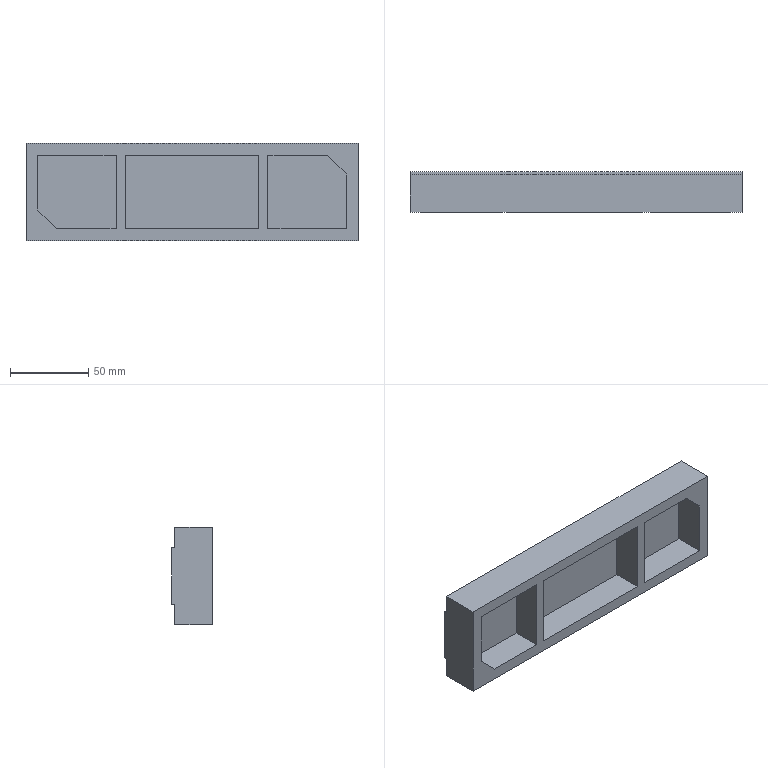Part | SolidWorks | features ICE 2, Extrusion 1, Rib 1, Shell 1 | 1 solid | 27 faces | box 212 x 26 x 62 mm | volume 172526 mm3 | plane 27
STEP:
#1=CARTESIAN_POINT('',(-86.5,18.5,-23.5));
#2=VERTEX_POINT('',#1);
#3=CARTESIAN_POINT('',(-86.5,0.,-23.5));
#4=VERTEX_POINT('',#3);
#5=CARTESIAN_POINT('',(-86.5,500000.,-23.5));
#6=DIRECTION('',(0.,-1.,0.));
#7=VECTOR('',#6,1000.);
#8=LINE('',#5,#7);
#9=EDGE_CURVE('',#2,#4,#8,.T.);
#10=ORIENTED_EDGE('',*,*,#9,.T.);
#11=CARTESIAN_POINT('',(-48.5,0.,-23.5));
#12=VERTEX_POINT('',#11);
#13=CARTESIAN_POINT('',(0.,0.,-23.5));
#14=DIRECTION('',(-1.,0.,0.));
#15=VECTOR('',#14,1000.);
#16=LINE('',#13,#15);
#17=EDGE_CURVE('',#12,#4,#16,.T.);
#18=ORIENTED_EDGE('',*,*,#17,.F.);
#19=CARTESIAN_POINT('',(-48.5,18.5,-23.5));
#20=VERTEX_POINT('',#19);
#21=CARTESIAN_POINT('',(-48.5,0.,-23.5));
#22=DIRECTION('',(0.,1.,0.));
#23=VECTOR('',#22,1000.);
#24=LINE('',#21,#23);
#25=EDGE_CURVE('',#12,#20,#24,.T.);
#26=ORIENTED_EDGE('',*,*,#25,.T.);
#27=CARTESIAN_POINT('',(0.,18.5,-23.5));
#28=DIRECTION('',(-1.,0.,0.));
#29=VECTOR('',#28,1000.);
#30=LINE('',#27,#29);
#31=EDGE_CURVE('',#20,#2,#30,.T.);
#32=ORIENTED_EDGE('',*,*,#31,.T.);
#33=EDGE_LOOP('',(#10,#18,#26,#32));
#34=FACE_OUTER_BOUND('',#33,.T.);
#35=CARTESIAN_POINT('',(-106.,26.,-23.5));
#36=DIRECTION('',(0.,0.,1.));
#37=DIRECTION('',(1.,0.,0.));
#38=AXIS2_PLACEMENT_3D('',#35,#36,#37);
#39=PLANE('',#38);
#40=ADVANCED_FACE('',(#34),#39,.T.);
#41=CARTESIAN_POINT('',(-98.5,18.5,23.5));
#42=VERTEX_POINT('',#41);
#43=CARTESIAN_POINT('',(-48.5,18.5,23.5));
#44=VERTEX_POINT('',#43);
#45=CARTESIAN_POINT('',(0.,18.5,23.5));
#46=DIRECTION('',(1.,0.,0.));
#47=VECTOR('',#46,1000.);
#48=LINE('',#45,#47);
#49=EDGE_CURVE('',#42,#44,#48,.T.);
#50=ORIENTED_EDGE('',*,*,#49,.T.);
#51=CARTESIAN_POINT('',(-48.5,0.,23.5));
#52=VERTEX_POINT('',#51);
#53=CARTESIAN_POINT('',(-48.5,26.,23.5));
#54=DIRECTION('',(0.,-1.,0.));
#55=VECTOR('',#54,1000.);
#56=LINE('',#53,#55);
#57=EDGE_CURVE('',#44,#52,#56,.T.);
#58=ORIENTED_EDGE('',*,*,#57,.T.);
#59=CARTESIAN_POINT('',(-98.5,0.,23.5));
#60=VERTEX_POINT('',#59);
#61=CARTESIAN_POINT('',(0.,0.,23.5));
#62=DIRECTION('',(1.,0.,0.));
#63=VECTOR('',#62,1000.);
#64=LINE('',#61,#63);
#65=EDGE_CURVE('',#60,#52,#64,.T.);
#66=ORIENTED_EDGE('',*,*,#65,.F.);
#67=CARTESIAN_POINT('',(-98.5,26.,23.5));
#68=DIRECTION('',(0.,-1.,0.));
#69=VECTOR('',#68,1000.);
#70=LINE('',#67,#69);
#71=EDGE_CURVE('',#42,#60,#70,.T.);
#72=ORIENTED_EDGE('',*,*,#71,.F.);
#73=EDGE_LOOP('',(#50,#58,#66,#72));
#74=FACE_OUTER_BOUND('',#73,.T.);
#75=CARTESIAN_POINT('',(-106.,26.,23.5));
#76=DIRECTION('',(0.,0.,-1.));
#77=DIRECTION('',(-1.,0.,0.));
#78=AXIS2_PLACEMENT_3D('',#75,#76,#77);
#79=PLANE('',#78);
#80=ADVANCED_FACE('',(#74),#79,.T.);
#81=CARTESIAN_POINT('',(-98.5,18.5,-11.5));
#82=VERTEX_POINT('',#81);
#83=CARTESIAN_POINT('',(-98.5,18.5,-11.5));
#84=DIRECTION('',(0.7071,0.,-0.7071));
#85=VECTOR('',#84,1000.);
#86=LINE('',#83,#85);
#87=EDGE_CURVE('',#82,#2,#86,.T.);
#88=ORIENTED_EDGE('',*,*,#87,.T.);
#89=ORIENTED_EDGE('',*,*,#31,.F.);
#90=CARTESIAN_POINT('',(-48.5,18.5,0.));
#91=DIRECTION('',(0.,0.,1.));
#92=VECTOR('',#91,1000.);
#93=LINE('',#90,#92);
#94=EDGE_CURVE('',#20,#44,#93,.T.);
#95=ORIENTED_EDGE('',*,*,#94,.T.);
#96=ORIENTED_EDGE('',*,*,#49,.F.);
#97=CARTESIAN_POINT('',(-98.5,18.5,0.));
#98=DIRECTION('',(0.,0.,1.));
#99=VECTOR('',#98,1000.);
#100=LINE('',#97,#99);
#101=EDGE_CURVE('',#82,#42,#100,.T.);
#102=ORIENTED_EDGE('',*,*,#101,.F.);
#103=EDGE_LOOP('',(#88,#89,#95,#96,#102));
#104=FACE_OUTER_BOUND('',#103,.T.);
#105=CARTESIAN_POINT('',(0.,18.5,0.));
#106=DIRECTION('',(0.,-1.,0.));
#107=DIRECTION('',(0.,0.,-1.));
#108=AXIS2_PLACEMENT_3D('',#105,#106,#107);
#109=PLANE('',#108);
#110=ADVANCED_FACE('',(#104),#109,.T.);
#111=CARTESIAN_POINT('',(-42.5,0.,-23.5));
#112=VERTEX_POINT('',#111);
#113=CARTESIAN_POINT('',(-42.5,18.5,-23.5));
#114=VERTEX_POINT('',#113);
#115=CARTESIAN_POINT('',(-42.5,0.,-23.5));
#116=DIRECTION('',(0.,1.,0.));
#117=VECTOR('',#116,1000.);
#118=LINE('',#115,#117);
#119=EDGE_CURVE('',#112,#114,#118,.T.);
#120=ORIENTED_EDGE('',*,*,#119,.F.);
#121=CARTESIAN_POINT('',(42.5,0.,-23.5));
#122=VERTEX_POINT('',#121);
#123=CARTESIAN_POINT('',(0.,0.,-23.5));
#124=DIRECTION('',(-1.,0.,0.));
#125=VECTOR('',#124,1000.);
#126=LINE('',#123,#125);
#127=EDGE_CURVE('',#122,#112,#126,.T.);
#128=ORIENTED_EDGE('',*,*,#127,.F.);
#129=CARTESIAN_POINT('',(42.5,18.5,-23.5));
#130=VERTEX_POINT('',#129);
#131=CARTESIAN_POINT('',(42.5,0.,-23.5));
#132=DIRECTION('',(0.,1.,0.));
#133=VECTOR('',#132,1000.);
#134=LINE('',#131,#133);
#135=EDGE_CURVE('',#122,#130,#134,.T.);
#136=ORIENTED_EDGE('',*,*,#135,.T.);
#137=CARTESIAN_POINT('',(0.,18.5,-23.5));
#138=DIRECTION('',(-1.,0.,0.));
#139=VECTOR('',#138,1000.);
#140=LINE('',#137,#139);
#141=EDGE_CURVE('',#130,#114,#140,.T.);
#142=ORIENTED_EDGE('',*,*,#141,.T.);
#143=EDGE_LOOP('',(#120,#128,#136,#142));
#144=FACE_OUTER_BOUND('',#143,.T.);
#145=CARTESIAN_POINT('',(-106.,26.,-23.5));
#146=DIRECTION('',(0.,0.,1.));
#147=DIRECTION('',(1.,0.,0.));
#148=AXIS2_PLACEMENT_3D('',#145,#146,#147);
#149=PLANE('',#148);
#150=ADVANCED_FACE('',(#144),#149,.T.);
#151=CARTESIAN_POINT('',(-42.5,18.5,23.5));
#152=VERTEX_POINT('',#151);
#153=CARTESIAN_POINT('',(-42.5,0.,23.5));
#154=VERTEX_POINT('',#153);
#155=CARTESIAN_POINT('',(-42.5,26.,23.5));
#156=DIRECTION('',(0.,-1.,0.));
#157=VECTOR('',#156,1000.);
#158=LINE('',#155,#157);
#159=EDGE_CURVE('',#152,#154,#158,.T.);
#160=ORIENTED_EDGE('',*,*,#159,.F.);
#161=CARTESIAN_POINT('',(42.5,18.5,23.5));
#162=VERTEX_POINT('',#161);
#163=CARTESIAN_POINT('',(0.,18.5,23.5));
#164=DIRECTION('',(1.,0.,0.));
#165=VECTOR('',#164,1000.);
#166=LINE('',#163,#165);
#167=EDGE_CURVE('',#152,#162,#166,.T.);
#168=ORIENTED_EDGE('',*,*,#167,.T.);
#169=CARTESIAN_POINT('',(42.5,0.,23.5));
#170=VERTEX_POINT('',#169);
#171=CARTESIAN_POINT('',(42.5,0.,23.5));
#172=DIRECTION('',(0.,1.,0.));
#173=VECTOR('',#172,1000.);
#174=LINE('',#171,#173);
#175=EDGE_CURVE('',#170,#162,#174,.T.);
#176=ORIENTED_EDGE('',*,*,#175,.F.);
#177=CARTESIAN_POINT('',(0.,0.,23.5));
#178=DIRECTION('',(1.,0.,0.));
#179=VECTOR('',#178,1000.);
#180=LINE('',#177,#179);
#181=EDGE_CURVE('',#154,#170,#180,.T.);
#182=ORIENTED_EDGE('',*,*,#181,.F.);
#183=EDGE_LOOP('',(#160,#168,#176,#182));
#184=FACE_OUTER_BOUND('',#183,.T.);
#185=CARTESIAN_POINT('',(-106.,26.,23.5));
#186=DIRECTION('',(0.,0.,-1.));
#187=DIRECTION('',(-1.,0.,0.));
#188=AXIS2_PLACEMENT_3D('',#185,#186,#187);
#189=PLANE('',#188);
#190=ADVANCED_FACE('',(#184),#189,.T.);
#191=CARTESIAN_POINT('',(-42.5,18.5,0.));
#192=DIRECTION('',(0.,0.,1.));
#193=VECTOR('',#192,1000.);
#194=LINE('',#191,#193);
#195=EDGE_CURVE('',#114,#152,#194,.T.);
#196=ORIENTED_EDGE('',*,*,#195,.F.);
#197=ORIENTED_EDGE('',*,*,#141,.F.);
#198=CARTESIAN_POINT('',(42.5,18.5,0.));
#199=DIRECTION('',(0.,0.,1.));
#200=VECTOR('',#199,1000.);
#201=LINE('',#198,#200);
#202=EDGE_CURVE('',#130,#162,#201,.T.);
#203=ORIENTED_EDGE('',*,*,#202,.T.);
#204=ORIENTED_EDGE('',*,*,#167,.F.);
#205=EDGE_LOOP('',(#196,#197,#203,#204));
#206=FACE_OUTER_BOUND('',#205,.T.);
#207=CARTESIAN_POINT('',(0.,18.5,0.));
#208=DIRECTION('',(0.,-1.,0.));
#209=DIRECTION('',(0.,0.,-1.));
#210=AXIS2_PLACEMENT_3D('',#207,#208,#209);
#211=PLANE('',#210);
#212=ADVANCED_FACE('',(#206),#211,.T.);
#213=CARTESIAN_POINT('',(106.,26.,18.));
#214=VERTEX_POINT('',#213);
#215=CARTESIAN_POINT('',(106.,26.,-18.));
#216=VERTEX_POINT('',#215);
#217=CARTESIAN_POINT('',(106.,26.,31.));
#218=DIRECTION('',(0.,0.,-1.));
#219=VECTOR('',#218,1000.);
#220=LINE('',#217,#219);
#221=EDGE_CURVE('',#214,#216,#220,.T.);
#222=ORIENTED_EDGE('',*,*,#221,.F.);
#223=CARTESIAN_POINT('',(106.,24.,18.));
#224=VERTEX_POINT('',#223);
#225=CARTESIAN_POINT('',(106.,24.,18.));
#226=DIRECTION('',(0.,1.,0.));
#227=VECTOR('',#226,1000.);
#228=LINE('',#225,#227);
#229=EDGE_CURVE('',#224,#214,#228,.T.);
#230=ORIENTED_EDGE('',*,*,#229,.F.);
#231=CARTESIAN_POINT('',(106.,24.,31.));
#232=VERTEX_POINT('',#231);
#233=CARTESIAN_POINT('',(106.,24.,31.));
#234=DIRECTION('',(0.,0.,-1.));
#235=VECTOR('',#234,1000.);
#236=LINE('',#233,#235);
#237=EDGE_CURVE('',#232,#224,#236,.T.);
#238=ORIENTED_EDGE('',*,*,#237,.F.);
#239=CARTESIAN_POINT('',(106.,0.,31.));
#240=VERTEX_POINT('',#239);
#241=CARTESIAN_POINT('',(106.,26.,31.));
#242=DIRECTION('',(0.,-1.,0.));
#243=VECTOR('',#242,1000.);
#244=LINE('',#241,#243);
#245=EDGE_CURVE('',#232,#240,#244,.T.);
#246=ORIENTED_EDGE('',*,*,#245,.T.);
#247=CARTESIAN_POINT('',(106.,0.,-31.));
#248=VERTEX_POINT('',#247);
#249=CARTESIAN_POINT('',(106.,0.,31.));
#250=DIRECTION('',(0.,0.,-1.));
#251=VECTOR('',#250,1000.);
#252=LINE('',#249,#251);
#253=EDGE_CURVE('',#240,#248,#252,.T.);
#254=ORIENTED_EDGE('',*,*,#253,.T.);
#255=CARTESIAN_POINT('',(106.,24.,-31.));
#256=VERTEX_POINT('',#255);
#257=CARTESIAN_POINT('',(106.,26.,-31.));
#258=DIRECTION('',(0.,-1.,0.));
#259=VECTOR('',#258,1000.);
#260=LINE('',#257,#259);
#261=EDGE_CURVE('',#256,#248,#260,.T.);
#262=ORIENTED_EDGE('',*,*,#261,.F.);
#263=CARTESIAN_POINT('',(106.,24.,-18.));
#264=VERTEX_POINT('',#263);
#265=CARTESIAN_POINT('',(106.,24.,-31.));
#266=DIRECTION('',(0.,0.,1.));
#267=VECTOR('',#266,1000.);
#268=LINE('',#265,#267);
#269=EDGE_CURVE('',#256,#264,#268,.T.);
#270=ORIENTED_EDGE('',*,*,#269,.T.);
#271=CARTESIAN_POINT('',(106.,24.,-18.));
#272=DIRECTION('',(0.,1.,0.));
#273=VECTOR('',#272,1000.);
#274=LINE('',#271,#273);
#275=EDGE_CURVE('',#264,#216,#274,.T.);
#276=ORIENTED_EDGE('',*,*,#275,.T.);
#277=EDGE_LOOP('',(#222,#230,#238,#246,#254,#262,#270,#276));
#278=FACE_OUTER_BOUND('',#277,.T.);
#279=CARTESIAN_POINT('',(106.,26.,31.));
#280=DIRECTION('',(-1.,0.,0.));
#281=DIRECTION('',(0.,0.,1.));
#282=AXIS2_PLACEMENT_3D('',#279,#280,#281);
#283=PLANE('',#282);
#284=ADVANCED_FACE('',(#278),#283,.F.);
#285=CARTESIAN_POINT('',(-106.,0.,-31.));
#286=VERTEX_POINT('',#285);
#287=CARTESIAN_POINT('',(-106.,0.,-31.));
#288=DIRECTION('',(-1.,0.,0.));
#289=VECTOR('',#288,1000.);
#290=LINE('',#287,#289);
#291=EDGE_CURVE('',#248,#286,#290,.T.);
#292=ORIENTED_EDGE('',*,*,#291,.T.);
#293=CARTESIAN_POINT('',(-106.,24.,-31.));
#294=VERTEX_POINT('',#293);
#295=CARTESIAN_POINT('',(-106.,26.,-31.));
#296=DIRECTION('',(0.,-1.,0.));
#297=VECTOR('',#296,1000.);
#298=LINE('',#295,#297);
#299=EDGE_CURVE('',#294,#286,#298,.T.);
#300=ORIENTED_EDGE('',*,*,#299,.F.);
#301=CARTESIAN_POINT('',(-106.,24.,-31.));
#302=DIRECTION('',(1.,0.,0.));
#303=VECTOR('',#302,1000.);
#304=LINE('',#301,#303);
#305=EDGE_CURVE('',#294,#256,#304,.T.);
#306=ORIENTED_EDGE('',*,*,#305,.T.);
#307=ORIENTED_EDGE('',*,*,#261,.T.);
#308=EDGE_LOOP('',(#292,#300,#306,#307));
#309=FACE_OUTER_BOUND('',#308,.T.);
#310=CARTESIAN_POINT('',(-106.,26.,-31.));
#311=DIRECTION('',(0.,0.,1.));
#312=DIRECTION('',(1.,0.,0.));
#313=AXIS2_PLACEMENT_3D('',#310,#311,#312);
#314=PLANE('',#313);
#315=ADVANCED_FACE('',(#309),#314,.F.);
#316=CARTESIAN_POINT('',(-106.,24.,31.));
#317=VERTEX_POINT('',#316);
#318=CARTESIAN_POINT('',(-106.,24.,18.));
#319=VERTEX_POINT('',#318);
#320=CARTESIAN_POINT('',(-106.,24.,31.));
#321=DIRECTION('',(0.,0.,-1.));
#322=VECTOR('',#321,1000.);
#323=LINE('',#320,#322);
#324=EDGE_CURVE('',#317,#319,#323,.T.);
#325=ORIENTED_EDGE('',*,*,#324,.T.);
#326=CARTESIAN_POINT('',(-106.,26.,18.));
#327=VERTEX_POINT('',#326);
#328=CARTESIAN_POINT('',(-106.,24.,18.));
#329=DIRECTION('',(0.,1.,0.));
#330=VECTOR('',#329,1000.);
#331=LINE('',#328,#330);
#332=EDGE_CURVE('',#319,#327,#331,.T.);
#333=ORIENTED_EDGE('',*,*,#332,.T.);
#334=CARTESIAN_POINT('',(-106.,26.,-18.));
#335=VERTEX_POINT('',#334);
#336=CARTESIAN_POINT('',(-106.,26.,31.));
#337=DIRECTION('',(0.,0.,1.));
#338=VECTOR('',#337,1000.);
#339=LINE('',#336,#338);
#340=EDGE_CURVE('',#335,#327,#339,.T.);
#341=ORIENTED_EDGE('',*,*,#340,.F.);
#342=CARTESIAN_POINT('',(-106.,24.,-18.));
#343=VERTEX_POINT('',#342);
#344=CARTESIAN_POINT('',(-106.,24.,-18.));
#345=DIRECTION('',(0.,1.,0.));
#346=VECTOR('',#345,1000.);
#347=LINE('',#344,#346);
#348=EDGE_CURVE('',#343,#335,#347,.T.);
#349=ORIENTED_EDGE('',*,*,#348,.F.);
#350=CARTESIAN_POINT('',(-106.,24.,-31.));
#351=DIRECTION('',(0.,0.,1.));
#352=VECTOR('',#351,1000.);
#353=LINE('',#350,#352);
#354=EDGE_CURVE('',#294,#343,#353,.T.);
#355=ORIENTED_EDGE('',*,*,#354,.F.);
#356=ORIENTED_EDGE('',*,*,#299,.T.);
#357=CARTESIAN_POINT('',(-106.,0.,31.));
#358=VERTEX_POINT('',#357);
#359=CARTESIAN_POINT('',(-106.,0.,31.));
#360=DIRECTION('',(0.,0.,1.));
#361=VECTOR('',#360,1000.);
#362=LINE('',#359,#361);
#363=EDGE_CURVE('',#286,#358,#362,.T.);
#364=ORIENTED_EDGE('',*,*,#363,.T.);
#365=CARTESIAN_POINT('',(-106.,26.,31.));
#366=DIRECTION('',(0.,-1.,0.));
#367=VECTOR('',#366,1000.);
#368=LINE('',#365,#367);
#369=EDGE_CURVE('',#317,#358,#368,.T.);
#370=ORIENTED_EDGE('',*,*,#369,.F.);
#371=EDGE_LOOP('',(#325,#333,#341,#349,#355,#356,#364,#370));
#372=FACE_OUTER_BOUND('',#371,.T.);
#373=CARTESIAN_POINT('',(-106.,26.,31.));
#374=DIRECTION('',(1.,0.,0.));
#375=DIRECTION('',(0.,0.,-1.));
#376=AXIS2_PLACEMENT_3D('',#373,#374,#375);
#377=PLANE('',#376);
#378=ADVANCED_FACE('',(#372),#377,.F.);
#379=ORIENTED_EDGE('',*,*,#221,.T.);
#380=CARTESIAN_POINT('',(-106.,26.,-18.));
#381=DIRECTION('',(1.,0.,0.));
#382=VECTOR('',#381,1000.);
#383=LINE('',#380,#382);
#384=EDGE_CURVE('',#335,#216,#383,.T.);
#385=ORIENTED_EDGE('',*,*,#384,.F.);
#386=ORIENTED_EDGE('',*,*,#340,.T.);
#387=CARTESIAN_POINT('',(-106.,26.,18.));
#388=DIRECTION('',(1.,0.,0.));
#389=VECTOR('',#388,1000.);
#390=LINE('',#387,#389);
#391=EDGE_CURVE('',#327,#214,#390,.T.);
#392=ORIENTED_EDGE('',*,*,#391,.T.);
#393=EDGE_LOOP('',(#379,#385,#386,#392));
#394=FACE_OUTER_BOUND('',#393,.T.);
#395=CARTESIAN_POINT('',(0.,26.,0.));
#396=DIRECTION('',(0.,-1.,0.));
#397=DIRECTION('',(0.,0.,-1.));
#398=AXIS2_PLACEMENT_3D('',#395,#396,#397);
#399=PLANE('',#398);
#400=ADVANCED_FACE('',(#394),#399,.F.);
#401=ORIENTED_EDGE('',*,*,#17,.T.);
#402=CARTESIAN_POINT('',(-98.5,0.,-11.5));
#403=VERTEX_POINT('',#402);
#404=CARTESIAN_POINT('',(-98.5,0.,-11.5));
#405=DIRECTION('',(-0.7071,0.,0.7071));
#406=VECTOR('',#405,1000.);
#407=LINE('',#404,#406);
#408=EDGE_CURVE('',#4,#403,#407,.T.);
#409=ORIENTED_EDGE('',*,*,#408,.T.);
#410=CARTESIAN_POINT('',(-98.5,0.,0.));
#411=DIRECTION('',(0.,0.,1.));
#412=VECTOR('',#411,1000.);
#413=LINE('',#410,#412);
#414=EDGE_CURVE('',#403,#60,#413,.T.);
#415=ORIENTED_EDGE('',*,*,#414,.T.);
#416=ORIENTED_EDGE('',*,*,#65,.T.);
#417=CARTESIAN_POINT('',(-48.5,0.,23.516));
#418=DIRECTION('',(0.,0.,-1.));
#419=VECTOR('',#418,1000.);
#420=LINE('',#417,#419);
#421=EDGE_CURVE('',#52,#12,#420,.T.);
#422=ORIENTED_EDGE('',*,*,#421,.T.);
#423=EDGE_LOOP('',(#401,#409,#415,#416,#422));
#424=FACE_BOUND('',#423,.T.);
#425=CARTESIAN_POINT('',(86.5,0.,23.5));
#426=VERTEX_POINT('',#425);
#427=CARTESIAN_POINT('',(98.5,0.,11.5));
#428=VERTEX_POINT('',#427);
#429=CARTESIAN_POINT('',(86.5,0.,23.5));
#430=DIRECTION('',(0.7071,0.,-0.7071));
#431=VECTOR('',#430,1000.);
#432=LINE('',#429,#431);
#433=EDGE_CURVE('',#426,#428,#432,.T.);
#434=ORIENTED_EDGE('',*,*,#433,.T.);
#435=CARTESIAN_POINT('',(98.5,0.,-23.5));
#436=VERTEX_POINT('',#435);
#437=CARTESIAN_POINT('',(98.5,0.,0.));
#438=DIRECTION('',(0.,0.,-1.));
#439=VECTOR('',#438,1000.);
#440=LINE('',#437,#439);
#441=EDGE_CURVE('',#428,#436,#440,.T.);
#442=ORIENTED_EDGE('',*,*,#441,.T.);
#443=CARTESIAN_POINT('',(48.5,0.,-23.5));
#444=VERTEX_POINT('',#443);
#445=CARTESIAN_POINT('',(0.,0.,-23.5));
#446=DIRECTION('',(-1.,0.,0.));
#447=VECTOR('',#446,1000.);
#448=LINE('',#445,#447);
#449=EDGE_CURVE('',#436,#444,#448,.T.);
#450=ORIENTED_EDGE('',*,*,#449,.T.);
#451=CARTESIAN_POINT('',(48.5,0.,23.5));
#452=VERTEX_POINT('',#451);
#453=CARTESIAN_POINT('',(48.5,0.,23.5));
#454=DIRECTION('',(0.,0.,-1.));
#455=VECTOR('',#454,1000.);
#456=LINE('',#453,#455);
#457=EDGE_CURVE('',#452,#444,#456,.T.);
#458=ORIENTED_EDGE('',*,*,#457,.F.);
#459=CARTESIAN_POINT('',(0.,0.,23.5));
#460=DIRECTION('',(1.,0.,0.));
#461=VECTOR('',#460,1000.);
#462=LINE('',#459,#461);
#463=EDGE_CURVE('',#452,#426,#462,.T.);
#464=ORIENTED_EDGE('',*,*,#463,.T.);
#465=EDGE_LOOP('',(#434,#442,#450,#458,#464));
#466=FACE_BOUND('',#465,.T.);
#467=ORIENTED_EDGE('',*,*,#253,.F.);
#468=CARTESIAN_POINT('',(-106.,0.,31.));
#469=DIRECTION('',(1.,0.,0.));
#470=VECTOR('',#469,1000.);
#471=LINE('',#468,#470);
#472=EDGE_CURVE('',#358,#240,#471,.T.);
#473=ORIENTED_EDGE('',*,*,#472,.F.);
#474=ORIENTED_EDGE('',*,*,#363,.F.);
#475=ORIENTED_EDGE('',*,*,#291,.F.);
#476=EDGE_LOOP('',(#467,#473,#474,#475));
#477=FACE_OUTER_BOUND('',#476,.T.);
#478=CARTESIAN_POINT('',(-42.5,0.,23.516));
#479=DIRECTION('',(0.,0.,-1.));
#480=VECTOR('',#479,1000.);
#481=LINE('',#478,#480);
#482=EDGE_CURVE('',#154,#112,#481,.T.);
#483=ORIENTED_EDGE('',*,*,#482,.F.);
#484=ORIENTED_EDGE('',*,*,#181,.T.);
#485=CARTESIAN_POINT('',(42.5,0.,23.5));
#486=DIRECTION('',(0.,0.,-1.));
#487=VECTOR('',#486,1000.);
#488=LINE('',#485,#487);
#489=EDGE_CURVE('',#170,#122,#488,.T.);
#490=ORIENTED_EDGE('',*,*,#489,.T.);
#491=ORIENTED_EDGE('',*,*,#127,.T.);
#492=EDGE_LOOP('',(#483,#484,#490,#491));
#493=FACE_BOUND('',#492,.T.);
#494=CARTESIAN_POINT('',(0.,0.,0.));
#495=DIRECTION('',(0.,-1.,0.));
#496=DIRECTION('',(0.,0.,-1.));
#497=AXIS2_PLACEMENT_3D('',#494,#495,#496);
#498=PLANE('',#497);
#499=ADVANCED_FACE('',(#424,#466,#477,#493),#498,.T.);
#500=ORIENTED_EDGE('',*,*,#472,.T.);
#501=ORIENTED_EDGE('',*,*,#245,.F.);
#502=CARTESIAN_POINT('',(-106.,24.,31.));
#503=DIRECTION('',(1.,0.,0.));
#504=VECTOR('',#503,1000.);
#505=LINE('',#502,#504);
#506=EDGE_CURVE('',#317,#232,#505,.T.);
#507=ORIENTED_EDGE('',*,*,#506,.F.);
#508=ORIENTED_EDGE('',*,*,#369,.T.);
#509=EDGE_LOOP('',(#500,#501,#507,#508));
#510=FACE_OUTER_BOUND('',#509,.T.);
#511=CARTESIAN_POINT('',(-106.,26.,31.));
#512=DIRECTION('',(0.,0.,-1.));
#513=DIRECTION('',(-1.,0.,0.));
#514=AXIS2_PLACEMENT_3D('',#511,#512,#513);
#515=PLANE('',#514);
#516=ADVANCED_FACE('',(#510),#515,.F.);
#517=CARTESIAN_POINT('',(98.5,18.5,11.5));
#518=VERTEX_POINT('',#517);
#519=CARTESIAN_POINT('',(98.5,500000.,11.5));
#520=DIRECTION('',(0.,-1.,0.));
#521=VECTOR('',#520,1000.);
#522=LINE('',#519,#521);
#523=EDGE_CURVE('',#518,#428,#522,.T.);
#524=ORIENTED_EDGE('',*,*,#523,.F.);
#525=CARTESIAN_POINT('',(98.5,18.5,-23.5));
#526=VERTEX_POINT('',#525);
#527=CARTESIAN_POINT('',(98.5,18.5,0.));
#528=DIRECTION('',(0.,0.,-1.));
#529=VECTOR('',#528,1000.);
#530=LINE('',#527,#529);
#531=EDGE_CURVE('',#518,#526,#530,.T.);
#532=ORIENTED_EDGE('',*,*,#531,.T.);
#533=CARTESIAN_POINT('',(98.5,26.,-23.5));
#534=DIRECTION('',(0.,-1.,0.));
#535=VECTOR('',#534,1000.);
#536=LINE('',#533,#535);
#537=EDGE_CURVE('',#526,#436,#536,.T.);
#538=ORIENTED_EDGE('',*,*,#537,.T.);
#539=ORIENTED_EDGE('',*,*,#441,.F.);
#540=EDGE_LOOP('',(#524,#532,#538,#539));
#541=FACE_OUTER_BOUND('',#540,.T.);
#542=CARTESIAN_POINT('',(98.5,26.,31.));
#543=DIRECTION('',(-1.,0.,0.));
#544=DIRECTION('',(0.,0.,1.));
#545=AXIS2_PLACEMENT_3D('',#542,#543,#544);
#546=PLANE('',#545);
#547=ADVANCED_FACE('',(#541),#546,.T.);
#548=CARTESIAN_POINT('',(48.5,18.5,-23.5));
#549=VERTEX_POINT('',#548);
#550=CARTESIAN_POINT('',(48.5,0.,-23.5));
#551=DIRECTION('',(0.,1.,0.));
#552=VECTOR('',#551,1000.);
#553=LINE('',#550,#552);
#554=EDGE_CURVE('',#444,#549,#553,.T.);
#555=ORIENTED_EDGE('',*,*,#554,.F.);
#556=ORIENTED_EDGE('',*,*,#449,.F.);
#557=ORIENTED_EDGE('',*,*,#537,.F.);
#558=CARTESIAN_POINT('',(0.,18.5,-23.5));
#559=DIRECTION('',(-1.,0.,0.));
#560=VECTOR('',#559,1000.);
#561=LINE('',#558,#560);
#562=EDGE_CURVE('',#526,#549,#561,.T.);
#563=ORIENTED_EDGE('',*,*,#562,.T.);
#564=EDGE_LOOP('',(#555,#556,#557,#563));
#565=FACE_OUTER_BOUND('',#564,.T.);
#566=CARTESIAN_POINT('',(-106.,26.,-23.5));
#567=DIRECTION('',(0.,0.,1.));
#568=DIRECTION('',(1.,0.,0.));
#569=AXIS2_PLACEMENT_3D('',#566,#567,#568);
#570=PLANE('',#569);
#571=ADVANCED_FACE('',(#565),#570,.T.);
#572=CARTESIAN_POINT('',(-98.5,500000.,-11.5));
#573=DIRECTION('',(0.,-1.,0.));
#574=VECTOR('',#573,1000.);
#575=LINE('',#572,#574);
#576=EDGE_CURVE('',#82,#403,#575,.T.);
#577=ORIENTED_EDGE('',*,*,#576,.F.);
#578=ORIENTED_EDGE('',*,*,#101,.T.);
#579=ORIENTED_EDGE('',*,*,#71,.T.);
#580=ORIENTED_EDGE('',*,*,#414,.F.);
#581=EDGE_LOOP('',(#577,#578,#579,#580));
#582=FACE_OUTER_BOUND('',#581,.T.);
#583=CARTESIAN_POINT('',(-98.5,26.,31.));
#584=DIRECTION('',(1.,0.,0.));
#585=DIRECTION('',(0.,0.,-1.));
#586=AXIS2_PLACEMENT_3D('',#583,#584,#585);
#587=PLANE('',#586);
#588=ADVANCED_FACE('',(#582),#587,.T.);
#589=CARTESIAN_POINT('',(86.5,18.5,23.5));
#590=VERTEX_POINT('',#589);
#591=CARTESIAN_POINT('',(86.5,500000.,23.5));
#592=DIRECTION('',(0.,-1.,0.));
#593=VECTOR('',#592,1000.);
#594=LINE('',#591,#593);
#595=EDGE_CURVE('',#590,#426,#594,.T.);
#596=ORIENTED_EDGE('',*,*,#595,.T.);
#597=ORIENTED_EDGE('',*,*,#463,.F.);
#598=CARTESIAN_POINT('',(48.5,18.5,23.5));
#599=VERTEX_POINT('',#598);
#600=CARTESIAN_POINT('',(48.5,0.,23.5));
#601=DIRECTION('',(0.,1.,0.));
#602=VECTOR('',#601,1000.);
#603=LINE('',#600,#602);
#604=EDGE_CURVE('',#452,#599,#603,.T.);
#605=ORIENTED_EDGE('',*,*,#604,.T.);
#606=CARTESIAN_POINT('',(0.,18.5,23.5));
#607=DIRECTION('',(1.,0.,0.));
#608=VECTOR('',#607,1000.);
#609=LINE('',#606,#608);
#610=EDGE_CURVE('',#599,#590,#609,.T.);
#611=ORIENTED_EDGE('',*,*,#610,.T.);
#612=EDGE_LOOP('',(#596,#597,#605,#611));
#613=FACE_OUTER_BOUND('',#612,.T.);
#614=CARTESIAN_POINT('',(-106.,26.,23.5));
#615=DIRECTION('',(0.,0.,-1.));
#616=DIRECTION('',(-1.,0.,0.));
#617=AXIS2_PLACEMENT_3D('',#614,#615,#616);
#618=PLANE('',#617);
#619=ADVANCED_FACE('',(#613),#618,.T.);
#620=CARTESIAN_POINT('',(86.5,18.5,23.5));
#621=DIRECTION('',(-0.7071,0.,0.7071));
#622=VECTOR('',#621,1000.);
#623=LINE('',#620,#622);
#624=EDGE_CURVE('',#518,#590,#623,.T.);
#625=ORIENTED_EDGE('',*,*,#624,.T.);
#626=ORIENTED_EDGE('',*,*,#610,.F.);
#627=CARTESIAN_POINT('',(48.5,18.5,0.));
#628=DIRECTION('',(0.,0.,1.));
#629=VECTOR('',#628,1000.);
#630=LINE('',#627,#629);
#631=EDGE_CURVE('',#549,#599,#630,.T.);
#632=ORIENTED_EDGE('',*,*,#631,.F.);
#633=ORIENTED_EDGE('',*,*,#562,.F.);
#634=ORIENTED_EDGE('',*,*,#531,.F.);
#635=EDGE_LOOP('',(#625,#626,#632,#633,#634));
#636=FACE_OUTER_BOUND('',#635,.T.);
#637=CARTESIAN_POINT('',(0.,18.5,0.));
#638=DIRECTION('',(0.,-1.,0.));
#639=DIRECTION('',(0.,0.,-1.));
#640=AXIS2_PLACEMENT_3D('',#637,#638,#639);
#641=PLANE('',#640);
#642=ADVANCED_FACE('',(#636),#641,.T.);
#643=CARTESIAN_POINT('',(-106.,24.,-18.));
#644=DIRECTION('',(1.,0.,0.));
#645=VECTOR('',#644,1000.);
#646=LINE('',#643,#645);
#647=EDGE_CURVE('',#343,#264,#646,.T.);
#648=ORIENTED_EDGE('',*,*,#647,.T.);
#649=ORIENTED_EDGE('',*,*,#269,.F.);
#650=ORIENTED_EDGE('',*,*,#305,.F.);
#651=ORIENTED_EDGE('',*,*,#354,.T.);
#652=EDGE_LOOP('',(#648,#649,#650,#651));
#653=FACE_OUTER_BOUND('',#652,.T.);
#654=CARTESIAN_POINT('',(-106.,24.,-31.));
#655=DIRECTION('',(0.,1.,0.));
#656=DIRECTION('',(0.,0.,1.));
#657=AXIS2_PLACEMENT_3D('',#654,#655,#656);
#658=PLANE('',#657);
#659=ADVANCED_FACE('',(#653),#658,.T.);
#660=ORIENTED_EDGE('',*,*,#275,.F.);
#661=ORIENTED_EDGE('',*,*,#647,.F.);
#662=ORIENTED_EDGE('',*,*,#348,.T.);
#663=ORIENTED_EDGE('',*,*,#384,.T.);
#664=EDGE_LOOP('',(#660,#661,#662,#663));
#665=FACE_OUTER_BOUND('',#664,.T.);
#666=CARTESIAN_POINT('',(-106.,24.,-18.));
#667=DIRECTION('',(0.,0.,-1.));
#668=DIRECTION('',(0.,1.,0.));
#669=AXIS2_PLACEMENT_3D('',#666,#667,#668);
#670=PLANE('',#669);
#671=ADVANCED_FACE('',(#665),#670,.T.);
#672=ORIENTED_EDGE('',*,*,#229,.T.);
#673=ORIENTED_EDGE('',*,*,#391,.F.);
#674=ORIENTED_EDGE('',*,*,#332,.F.);
#675=CARTESIAN_POINT('',(-106.,24.,18.));
#676=DIRECTION('',(1.,0.,0.));
#677=VECTOR('',#676,1000.);
#678=LINE('',#675,#677);
#679=EDGE_CURVE('',#319,#224,#678,.T.);
#680=ORIENTED_EDGE('',*,*,#679,.T.);
#681=EDGE_LOOP('',(#672,#673,#674,#680));
#682=FACE_OUTER_BOUND('',#681,.T.);
#683=CARTESIAN_POINT('',(-106.,24.,18.));
#684=DIRECTION('',(0.,0.,-1.));
#685=DIRECTION('',(0.,1.,0.));
#686=AXIS2_PLACEMENT_3D('',#683,#684,#685);
#687=PLANE('',#686);
#688=ADVANCED_FACE('',(#682),#687,.F.);
#689=ORIENTED_EDGE('',*,*,#506,.T.);
#690=ORIENTED_EDGE('',*,*,#237,.T.);
#691=ORIENTED_EDGE('',*,*,#679,.F.);
#692=ORIENTED_EDGE('',*,*,#324,.F.);
#693=EDGE_LOOP('',(#689,#690,#691,#692));
#694=FACE_OUTER_BOUND('',#693,.T.);
#695=CARTESIAN_POINT('',(-106.,24.,31.));
#696=DIRECTION('',(0.,-1.,0.));
#697=DIRECTION('',(0.,0.,-1.));
#698=AXIS2_PLACEMENT_3D('',#695,#696,#697);
#699=PLANE('',#698);
#700=ADVANCED_FACE('',(#694),#699,.F.);
#701=ORIENTED_EDGE('',*,*,#554,.T.);
#702=ORIENTED_EDGE('',*,*,#631,.T.);
#703=ORIENTED_EDGE('',*,*,#604,.F.);
#704=ORIENTED_EDGE('',*,*,#457,.T.);
#705=EDGE_LOOP('',(#701,#702,#703,#704));
#706=FACE_OUTER_BOUND('',#705,.T.);
#707=CARTESIAN_POINT('',(48.5,0.,23.5));
#708=DIRECTION('',(1.,0.,0.));
#709=DIRECTION('',(0.,0.,-1.));
#710=AXIS2_PLACEMENT_3D('',#707,#708,#709);
#711=PLANE('',#710);
#712=ADVANCED_FACE('',(#706),#711,.T.);
#713=ORIENTED_EDGE('',*,*,#202,.F.);
#714=ORIENTED_EDGE('',*,*,#135,.F.);
#715=ORIENTED_EDGE('',*,*,#489,.F.);
#716=ORIENTED_EDGE('',*,*,#175,.T.);
#717=EDGE_LOOP('',(#713,#714,#715,#716));
#718=FACE_OUTER_BOUND('',#717,.T.);
#719=CARTESIAN_POINT('',(42.5,0.,23.5));
#720=DIRECTION('',(1.,0.,0.));
#721=DIRECTION('',(0.,0.,-1.));
#722=AXIS2_PLACEMENT_3D('',#719,#720,#721);
#723=PLANE('',#722);
#724=ADVANCED_FACE('',(#718),#723,.F.);
#725=ORIENTED_EDGE('',*,*,#195,.T.);
#726=ORIENTED_EDGE('',*,*,#159,.T.);
#727=ORIENTED_EDGE('',*,*,#482,.T.);
#728=ORIENTED_EDGE('',*,*,#119,.T.);
#729=EDGE_LOOP('',(#725,#726,#727,#728));
#730=FACE_OUTER_BOUND('',#729,.T.);
#731=CARTESIAN_POINT('',(-42.5,0.,23.516));
#732=DIRECTION('',(1.,0.,0.));
#733=DIRECTION('',(0.,0.,-1.));
#734=AXIS2_PLACEMENT_3D('',#731,#732,#733);
#735=PLANE('',#734);
#736=ADVANCED_FACE('',(#730),#735,.T.);
#737=ORIENTED_EDGE('',*,*,#57,.F.);
#738=ORIENTED_EDGE('',*,*,#94,.F.);
#739=ORIENTED_EDGE('',*,*,#25,.F.);
#740=ORIENTED_EDGE('',*,*,#421,.F.);
#741=EDGE_LOOP('',(#737,#738,#739,#740));
#742=FACE_OUTER_BOUND('',#741,.T.);
#743=CARTESIAN_POINT('',(-48.5,0.,23.516));
#744=DIRECTION('',(1.,0.,0.));
#745=DIRECTION('',(0.,0.,-1.));
#746=AXIS2_PLACEMENT_3D('',#743,#744,#745);
#747=PLANE('',#746);
#748=ADVANCED_FACE('',(#742),#747,.F.);
#749=ORIENTED_EDGE('',*,*,#624,.F.);
#750=ORIENTED_EDGE('',*,*,#523,.T.);
#751=ORIENTED_EDGE('',*,*,#433,.F.);
#752=ORIENTED_EDGE('',*,*,#595,.F.);
#753=EDGE_LOOP('',(#749,#750,#751,#752));
#754=FACE_OUTER_BOUND('',#753,.T.);
#755=CARTESIAN_POINT('',(86.5,500000.,23.5));
#756=DIRECTION('',(-0.7071,0.,-0.7071));
#757=DIRECTION('',(-0.7071,0.,0.7071));
#758=AXIS2_PLACEMENT_3D('',#755,#756,#757);
#759=PLANE('',#758);
#760=ADVANCED_FACE('',(#754),#759,.T.);
#761=ORIENTED_EDGE('',*,*,#87,.F.);
#762=ORIENTED_EDGE('',*,*,#576,.T.);
#763=ORIENTED_EDGE('',*,*,#408,.F.);
#764=ORIENTED_EDGE('',*,*,#9,.F.);
#765=EDGE_LOOP('',(#761,#762,#763,#764));
#766=FACE_OUTER_BOUND('',#765,.T.);
#767=CARTESIAN_POINT('',(-98.5,500000.,-11.5));
#768=DIRECTION('',(0.7071,0.,0.7071));
#769=DIRECTION('',(0.7071,0.,-0.7071));
#770=AXIS2_PLACEMENT_3D('',#767,#768,#769);
#771=PLANE('',#770);
#772=ADVANCED_FACE('',(#766),#771,.T.);
#773=CLOSED_SHELL('',(#40,#80,#110,#150,#190,#212,#284,#315,#378,#400,#499,#516,#547,#571,#588,#619,#642,#659,#671,#688,#700,#712,#724,#736,#748,#760,#772));
#774=MANIFOLD_SOLID_BREP('',#773);
#775=CARTESIAN_POINT('',(0.,0.,0.));
#776=DIRECTION('',(0.,0.,1.));
#777=DIRECTION('',(1.,0.,0.));
#778=AXIS2_PLACEMENT_3D('',#775,#776,#777);
#779=(LENGTH_UNIT()NAMED_UNIT(*)SI_UNIT(.MILLI.,.METRE.));
#780=UNCERTAINTY_MEASURE_WITH_UNIT(LENGTH_MEASURE(0.00001),#779,'','');
#781=(NAMED_UNIT(*)PLANE_ANGLE_UNIT()SI_UNIT($,.RADIAN.));
#782=(NAMED_UNIT(*)SI_UNIT($,.STERADIAN.)SOLID_ANGLE_UNIT());
#783=(GEOMETRIC_REPRESENTATION_CONTEXT(3)GLOBAL_UNCERTAINTY_ASSIGNED_CONTEXT((#780))GLOBAL_UNIT_ASSIGNED_CONTEXT((#779,#781,#782))REPRESENTATION_CONTEXT('',''));
#784=ADVANCED_BREP_SHAPE_REPRESENTATION('',(#774,#778),#783);